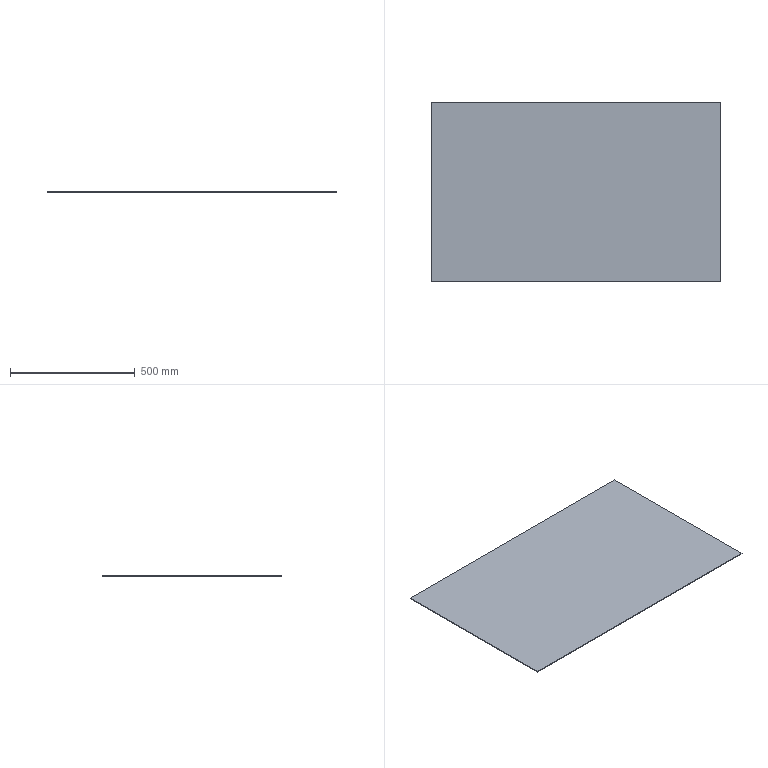Part | SolidWorks | features Extrusion 1 | 1 solid | 6 faces | box 1160 x 720 x 3 mm | volume 2505600 mm3 | plane 6
STEP:
#1=CARTESIAN_POINT('',(580.,-360.,0.));
#2=VERTEX_POINT('',#1);
#3=CARTESIAN_POINT('',(580.,360.,0.));
#4=VERTEX_POINT('',#3);
#5=CARTESIAN_POINT('',(580.,-360.,0.));
#6=DIRECTION('',(0.,1.,0.));
#7=VECTOR('',#6,1000.);
#8=LINE('',#5,#7);
#9=EDGE_CURVE('',#2,#4,#8,.T.);
#10=ORIENTED_EDGE('',*,*,#9,.T.);
#11=CARTESIAN_POINT('',(580.,360.,3.));
#12=VERTEX_POINT('',#11);
#13=CARTESIAN_POINT('',(580.,360.,3.));
#14=DIRECTION('',(0.,0.,-1.));
#15=VECTOR('',#14,1000.);
#16=LINE('',#13,#15);
#17=EDGE_CURVE('',#12,#4,#16,.T.);
#18=ORIENTED_EDGE('',*,*,#17,.F.);
#19=CARTESIAN_POINT('',(580.,-360.,3.));
#20=VERTEX_POINT('',#19);
#21=CARTESIAN_POINT('',(580.,-360.,3.));
#22=DIRECTION('',(0.,1.,0.));
#23=VECTOR('',#22,1000.);
#24=LINE('',#21,#23);
#25=EDGE_CURVE('',#20,#12,#24,.T.);
#26=ORIENTED_EDGE('',*,*,#25,.F.);
#27=CARTESIAN_POINT('',(580.,-360.,3.));
#28=DIRECTION('',(0.,0.,-1.));
#29=VECTOR('',#28,1000.);
#30=LINE('',#27,#29);
#31=EDGE_CURVE('',#20,#2,#30,.T.);
#32=ORIENTED_EDGE('',*,*,#31,.T.);
#33=EDGE_LOOP('',(#10,#18,#26,#32));
#34=FACE_OUTER_BOUND('',#33,.T.);
#35=CARTESIAN_POINT('',(580.,-360.,3.));
#36=DIRECTION('',(-1.,0.,0.));
#37=DIRECTION('',(0.,0.,1.));
#38=AXIS2_PLACEMENT_3D('',#35,#36,#37);
#39=PLANE('',#38);
#40=ADVANCED_FACE('',(#34),#39,.F.);
#41=CARTESIAN_POINT('',(-580.,360.,0.));
#42=VERTEX_POINT('',#41);
#43=CARTESIAN_POINT('',(-580.,360.,0.));
#44=DIRECTION('',(-1.,0.,0.));
#45=VECTOR('',#44,1000.);
#46=LINE('',#43,#45);
#47=EDGE_CURVE('',#4,#42,#46,.T.);
#48=ORIENTED_EDGE('',*,*,#47,.T.);
#49=CARTESIAN_POINT('',(-580.,360.,3.));
#50=VERTEX_POINT('',#49);
#51=CARTESIAN_POINT('',(-580.,360.,3.));
#52=DIRECTION('',(0.,0.,-1.));
#53=VECTOR('',#52,1000.);
#54=LINE('',#51,#53);
#55=EDGE_CURVE('',#50,#42,#54,.T.);
#56=ORIENTED_EDGE('',*,*,#55,.F.);
#57=CARTESIAN_POINT('',(-580.,360.,3.));
#58=DIRECTION('',(-1.,0.,0.));
#59=VECTOR('',#58,1000.);
#60=LINE('',#57,#59);
#61=EDGE_CURVE('',#12,#50,#60,.T.);
#62=ORIENTED_EDGE('',*,*,#61,.F.);
#63=ORIENTED_EDGE('',*,*,#17,.T.);
#64=EDGE_LOOP('',(#48,#56,#62,#63));
#65=FACE_OUTER_BOUND('',#64,.T.);
#66=CARTESIAN_POINT('',(-580.,360.,3.));
#67=DIRECTION('',(0.,-1.,0.));
#68=DIRECTION('',(0.,0.,-1.));
#69=AXIS2_PLACEMENT_3D('',#66,#67,#68);
#70=PLANE('',#69);
#71=ADVANCED_FACE('',(#65),#70,.F.);
#72=CARTESIAN_POINT('',(-580.,-360.,0.));
#73=VERTEX_POINT('',#72);
#74=CARTESIAN_POINT('',(-580.,-360.,0.));
#75=DIRECTION('',(0.,-1.,0.));
#76=VECTOR('',#75,1000.);
#77=LINE('',#74,#76);
#78=EDGE_CURVE('',#42,#73,#77,.T.);
#79=ORIENTED_EDGE('',*,*,#78,.T.);
#80=CARTESIAN_POINT('',(-580.,-360.,3.));
#81=VERTEX_POINT('',#80);
#82=CARTESIAN_POINT('',(-580.,-360.,3.));
#83=DIRECTION('',(0.,0.,-1.));
#84=VECTOR('',#83,1000.);
#85=LINE('',#82,#84);
#86=EDGE_CURVE('',#81,#73,#85,.T.);
#87=ORIENTED_EDGE('',*,*,#86,.F.);
#88=CARTESIAN_POINT('',(-580.,-360.,3.));
#89=DIRECTION('',(0.,-1.,0.));
#90=VECTOR('',#89,1000.);
#91=LINE('',#88,#90);
#92=EDGE_CURVE('',#50,#81,#91,.T.);
#93=ORIENTED_EDGE('',*,*,#92,.F.);
#94=ORIENTED_EDGE('',*,*,#55,.T.);
#95=EDGE_LOOP('',(#79,#87,#93,#94));
#96=FACE_OUTER_BOUND('',#95,.T.);
#97=CARTESIAN_POINT('',(-580.,-360.,3.));
#98=DIRECTION('',(1.,0.,0.));
#99=DIRECTION('',(0.,0.,-1.));
#100=AXIS2_PLACEMENT_3D('',#97,#98,#99);
#101=PLANE('',#100);
#102=ADVANCED_FACE('',(#96),#101,.F.);
#103=CARTESIAN_POINT('',(-580.,-360.,0.));
#104=DIRECTION('',(1.,0.,0.));
#105=VECTOR('',#104,1000.);
#106=LINE('',#103,#105);
#107=EDGE_CURVE('',#73,#2,#106,.T.);
#108=ORIENTED_EDGE('',*,*,#107,.T.);
#109=ORIENTED_EDGE('',*,*,#31,.F.);
#110=CARTESIAN_POINT('',(-580.,-360.,3.));
#111=DIRECTION('',(1.,0.,0.));
#112=VECTOR('',#111,1000.);
#113=LINE('',#110,#112);
#114=EDGE_CURVE('',#81,#20,#113,.T.);
#115=ORIENTED_EDGE('',*,*,#114,.F.);
#116=ORIENTED_EDGE('',*,*,#86,.T.);
#117=EDGE_LOOP('',(#108,#109,#115,#116));
#118=FACE_OUTER_BOUND('',#117,.T.);
#119=CARTESIAN_POINT('',(-580.,-360.,3.));
#120=DIRECTION('',(0.,1.,0.));
#121=DIRECTION('',(0.,0.,1.));
#122=AXIS2_PLACEMENT_3D('',#119,#120,#121);
#123=PLANE('',#122);
#124=ADVANCED_FACE('',(#118),#123,.F.);
#125=ORIENTED_EDGE('',*,*,#25,.T.);
#126=ORIENTED_EDGE('',*,*,#61,.T.);
#127=ORIENTED_EDGE('',*,*,#92,.T.);
#128=ORIENTED_EDGE('',*,*,#114,.T.);
#129=EDGE_LOOP('',(#125,#126,#127,#128));
#130=FACE_OUTER_BOUND('',#129,.T.);
#131=CARTESIAN_POINT('',(0.,0.,3.));
#132=DIRECTION('',(0.,0.,-1.));
#133=DIRECTION('',(-1.,0.,0.));
#134=AXIS2_PLACEMENT_3D('',#131,#132,#133);
#135=PLANE('',#134);
#136=ADVANCED_FACE('',(#130),#135,.F.);
#137=ORIENTED_EDGE('',*,*,#9,.F.);
#138=ORIENTED_EDGE('',*,*,#107,.F.);
#139=ORIENTED_EDGE('',*,*,#78,.F.);
#140=ORIENTED_EDGE('',*,*,#47,.F.);
#141=EDGE_LOOP('',(#137,#138,#139,#140));
#142=FACE_OUTER_BOUND('',#141,.T.);
#143=CARTESIAN_POINT('',(0.,0.,0.));
#144=DIRECTION('',(0.,0.,-1.));
#145=DIRECTION('',(-1.,0.,0.));
#146=AXIS2_PLACEMENT_3D('',#143,#144,#145);
#147=PLANE('',#146);
#148=ADVANCED_FACE('',(#142),#147,.T.);
#149=CLOSED_SHELL('',(#40,#71,#102,#124,#136,#148));
#150=MANIFOLD_SOLID_BREP('',#149);
#151=CARTESIAN_POINT('',(0.,0.,0.));
#152=DIRECTION('',(0.,0.,1.));
#153=DIRECTION('',(1.,0.,0.));
#154=AXIS2_PLACEMENT_3D('',#151,#152,#153);
#155=(LENGTH_UNIT()NAMED_UNIT(*)SI_UNIT(.MILLI.,.METRE.));
#156=UNCERTAINTY_MEASURE_WITH_UNIT(LENGTH_MEASURE(0.00001),#155,'','');
#157=(NAMED_UNIT(*)PLANE_ANGLE_UNIT()SI_UNIT($,.RADIAN.));
#158=(NAMED_UNIT(*)SI_UNIT($,.STERADIAN.)SOLID_ANGLE_UNIT());
#159=(GEOMETRIC_REPRESENTATION_CONTEXT(3)GLOBAL_UNCERTAINTY_ASSIGNED_CONTEXT((#156))GLOBAL_UNIT_ASSIGNED_CONTEXT((#155,#157,#158))REPRESENTATION_CONTEXT('',''));
#160=ADVANCED_BREP_SHAPE_REPRESENTATION('',(#150,#154),#159);